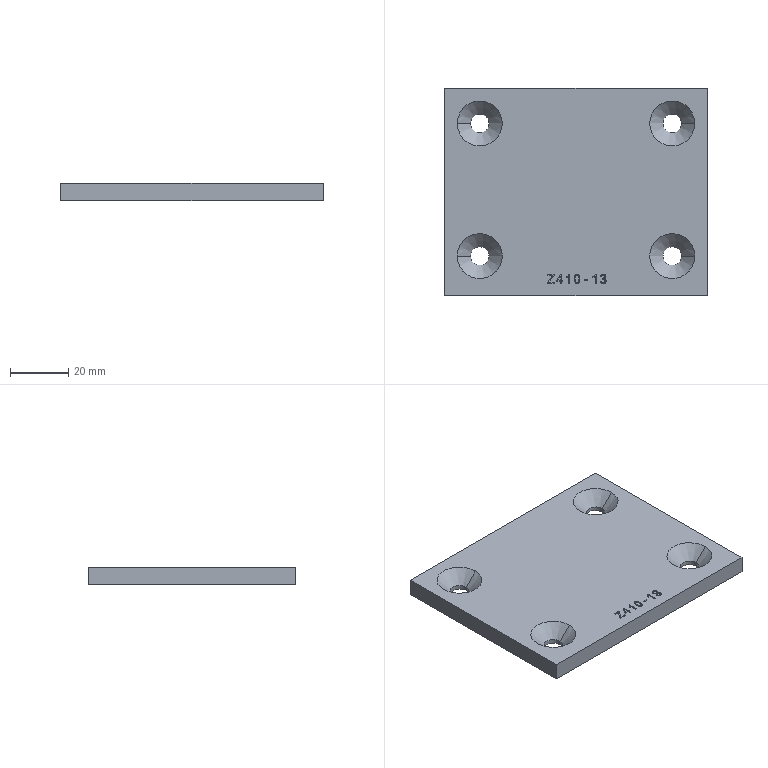Part | Creo | 1 solid | 129 faces | box 90 x 71 x 6 mm | volume 36357 mm3 | other 63 | plane 49 | cylinder 9 | cone 8 | commonest cylinder face diameters 6.4 x8 45.582 x1